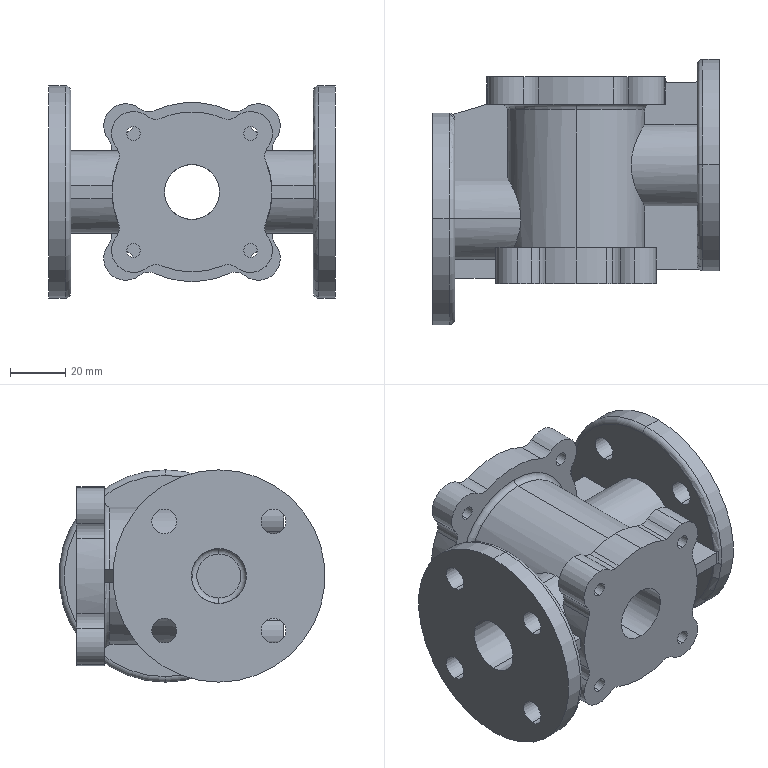Part | SolidWorks | features ICE 14, Fillet 9, Rib 4, 3DProfileFeature 2, HoleWzd 2, Chamfer 1, Extrusion 1, RevCut 1 | 1 solid | 186 faces | box 104 x 96.5 x 77 mm | volume 206017 mm3 | cylinder 112 | plane 41 | cone 18 | torus 15 | commonest cylinder face diameters 10 x20 5 x16 9 x16 16 x12 20 x10 30 x6